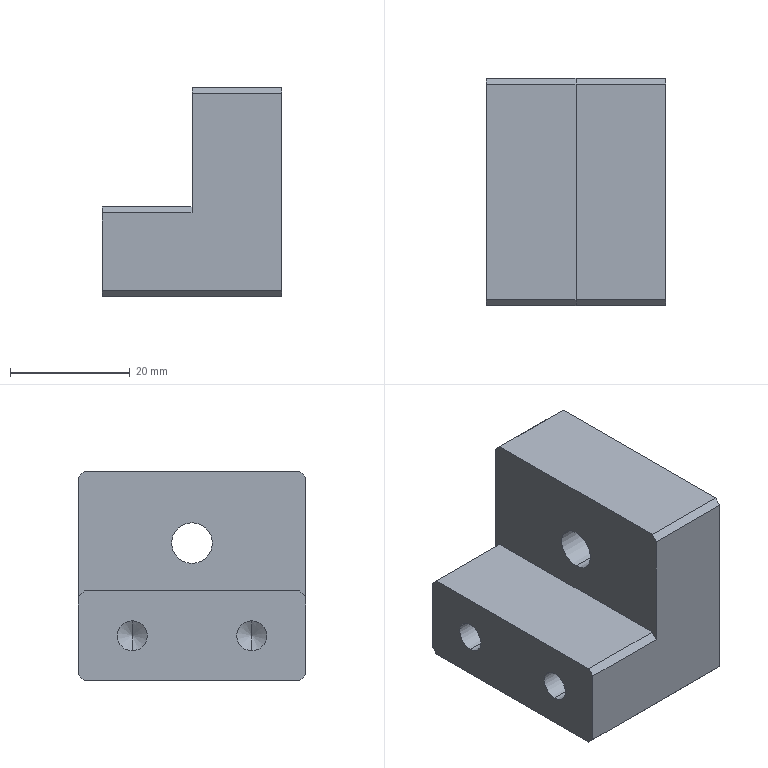Part | SolidWorks | features BaseBody 1 | 1 solid | 27 faces | box 30 x 38 x 35 mm | volume 26589 mm3 | plane 15 | cylinder 8 | cone 4 | commonest cylinder face diameters 5 x4 6.8 x2 18.5 x2
STEP:
#1=CARTESIAN_POINT('',(15.,0.,26.4));
#2=VERTEX_POINT('',#1);
#3=CARTESIAN_POINT('',(15.,0.,19.6));
#4=VERTEX_POINT('',#3);
#5=CARTESIAN_POINT('',(15.,0.,23.));
#6=DIRECTION('',(1.,0.,0.));
#7=DIRECTION('',(0.,0.,-1.));
#8=AXIS2_PLACEMENT_3D('',#5,#6,#7);
#9=CIRCLE('',#8,3.4);
#10=EDGE_CURVE('',#2,#4,#9,.T.);
#11=ORIENTED_EDGE('',*,*,#10,.F.);
#12=CARTESIAN_POINT('',(27.,0.,26.4));
#13=VERTEX_POINT('',#12);
#14=CARTESIAN_POINT('',(27.,0.,26.4));
#15=DIRECTION('',(1.,0.,0.));
#16=VECTOR('',#15,1000.);
#17=LINE('',#14,#16);
#18=EDGE_CURVE('',#2,#13,#17,.T.);
#19=ORIENTED_EDGE('',*,*,#18,.T.);
#20=CARTESIAN_POINT('',(27.,0.,19.6));
#21=VERTEX_POINT('',#20);
#22=CARTESIAN_POINT('',(27.,0.,23.));
#23=DIRECTION('',(1.,0.,0.));
#24=DIRECTION('',(0.,0.,-1.));
#25=AXIS2_PLACEMENT_3D('',#22,#23,#24);
#26=CIRCLE('',#25,3.4);
#27=EDGE_CURVE('',#13,#21,#26,.T.);
#28=ORIENTED_EDGE('',*,*,#27,.T.);
#29=CARTESIAN_POINT('',(27.,0.,19.6));
#30=DIRECTION('',(1.,0.,0.));
#31=VECTOR('',#30,1000.);
#32=LINE('',#29,#31);
#33=EDGE_CURVE('',#4,#21,#32,.T.);
#34=ORIENTED_EDGE('',*,*,#33,.F.);
#35=EDGE_LOOP('',(#11,#19,#28,#34));
#36=FACE_OUTER_BOUND('',#35,.T.);
#37=CARTESIAN_POINT('',(27.,0.,23.));
#38=DIRECTION('',(1.,0.,0.));
#39=DIRECTION('',(0.,0.,-1.));
#40=AXIS2_PLACEMENT_3D('',#37,#38,#39);
#41=CYLINDRICAL_SURFACE('',#40,3.4);
#42=ADVANCED_FACE('',(#36),#41,.F.);
#43=CARTESIAN_POINT('',(27.,0.,32.25));
#44=VERTEX_POINT('',#43);
#45=CARTESIAN_POINT('',(27.,0.,13.75));
#46=VERTEX_POINT('',#45);
#47=CARTESIAN_POINT('',(27.,0.,23.));
#48=DIRECTION('',(1.,0.,0.));
#49=DIRECTION('',(0.,0.,-1.));
#50=AXIS2_PLACEMENT_3D('',#47,#48,#49);
#51=CIRCLE('',#50,9.25);
#52=EDGE_CURVE('',#44,#46,#51,.T.);
#53=ORIENTED_EDGE('',*,*,#52,.F.);
#54=CARTESIAN_POINT('',(30.,0.,32.25));
#55=VERTEX_POINT('',#54);
#56=CARTESIAN_POINT('',(27.,0.,32.25));
#57=DIRECTION('',(1.,0.,0.));
#58=VECTOR('',#57,1000.);
#59=LINE('',#56,#58);
#60=EDGE_CURVE('',#44,#55,#59,.T.);
#61=ORIENTED_EDGE('',*,*,#60,.T.);
#62=CARTESIAN_POINT('',(30.,0.,13.75));
#63=VERTEX_POINT('',#62);
#64=CARTESIAN_POINT('',(30.,0.,23.));
#65=DIRECTION('',(1.,0.,0.));
#66=DIRECTION('',(0.,0.,-1.));
#67=AXIS2_PLACEMENT_3D('',#64,#65,#66);
#68=CIRCLE('',#67,9.25);
#69=EDGE_CURVE('',#55,#63,#68,.T.);
#70=ORIENTED_EDGE('',*,*,#69,.T.);
#71=CARTESIAN_POINT('',(27.,0.,13.75));
#72=DIRECTION('',(1.,0.,0.));
#73=VECTOR('',#72,1000.);
#74=LINE('',#71,#73);
#75=EDGE_CURVE('',#46,#63,#74,.T.);
#76=ORIENTED_EDGE('',*,*,#75,.F.);
#77=EDGE_LOOP('',(#53,#61,#70,#76));
#78=FACE_OUTER_BOUND('',#77,.T.);
#79=CARTESIAN_POINT('',(27.,0.,23.));
#80=DIRECTION('',(1.,0.,0.));
#81=DIRECTION('',(0.,0.,-1.));
#82=AXIS2_PLACEMENT_3D('',#79,#80,#81);
#83=CYLINDRICAL_SURFACE('',#82,9.25);
#84=ADVANCED_FACE('',(#78),#83,.F.);
#85=CARTESIAN_POINT('',(15.,10.,5.));
#86=VERTEX_POINT('',#85);
#87=CARTESIAN_POINT('',(15.,10.,10.));
#88=VERTEX_POINT('',#87);
#89=CARTESIAN_POINT('',(15.,10.,7.5));
#90=DIRECTION('',(-1.,0.,0.));
#91=DIRECTION('',(0.,0.,1.));
#92=AXIS2_PLACEMENT_3D('',#89,#90,#91);
#93=CIRCLE('',#92,2.5);
#94=EDGE_CURVE('',#86,#88,#93,.T.);
#95=ORIENTED_EDGE('',*,*,#94,.F.);
#96=CARTESIAN_POINT('',(0.,10.,5.));
#97=VERTEX_POINT('',#96);
#98=CARTESIAN_POINT('',(0.,10.,5.));
#99=DIRECTION('',(-1.,0.,0.));
#100=VECTOR('',#99,1000.);
#101=LINE('',#98,#100);
#102=EDGE_CURVE('',#86,#97,#101,.T.);
#103=ORIENTED_EDGE('',*,*,#102,.T.);
#104=CARTESIAN_POINT('',(0.,10.,10.));
#105=VERTEX_POINT('',#104);
#106=CARTESIAN_POINT('',(0.,10.,7.5));
#107=DIRECTION('',(-1.,0.,0.));
#108=DIRECTION('',(0.,0.,1.));
#109=AXIS2_PLACEMENT_3D('',#106,#107,#108);
#110=CIRCLE('',#109,2.5);
#111=EDGE_CURVE('',#97,#105,#110,.T.);
#112=ORIENTED_EDGE('',*,*,#111,.T.);
#113=CARTESIAN_POINT('',(0.,10.,10.));
#114=DIRECTION('',(-1.,0.,0.));
#115=VECTOR('',#114,1000.);
#116=LINE('',#113,#115);
#117=EDGE_CURVE('',#88,#105,#116,.T.);
#118=ORIENTED_EDGE('',*,*,#117,.F.);
#119=EDGE_LOOP('',(#95,#103,#112,#118));
#120=FACE_OUTER_BOUND('',#119,.T.);
#121=CARTESIAN_POINT('',(0.,10.,7.5));
#122=DIRECTION('',(-1.,0.,0.));
#123=DIRECTION('',(0.,0.,1.));
#124=AXIS2_PLACEMENT_3D('',#121,#122,#123);
#125=CYLINDRICAL_SURFACE('',#124,2.5);
#126=ADVANCED_FACE('',(#120),#125,.F.);
#127=CARTESIAN_POINT('',(16.502,10.,7.5));
#128=VERTEX_POINT('',#127);
#129=CARTESIAN_POINT('',(15.,10.,10.));
#130=DIRECTION('',(-0.515,0.,0.8572));
#131=VECTOR('',#130,1000.);
#132=LINE('',#129,#131);
#133=EDGE_CURVE('',#128,#88,#132,.T.);
#134=ORIENTED_EDGE('',*,*,#133,.F.);
#135=CARTESIAN_POINT('',(15.,10.,5.));
#136=DIRECTION('',(-0.515,0.,-0.8572));
#137=VECTOR('',#136,1000.);
#138=LINE('',#135,#137);
#139=EDGE_CURVE('',#128,#86,#138,.T.);
#140=ORIENTED_EDGE('',*,*,#139,.T.);
#141=ORIENTED_EDGE('',*,*,#94,.T.);
#142=EDGE_LOOP('',(#134,#140,#141));
#143=FACE_OUTER_BOUND('',#142,.T.);
#144=CARTESIAN_POINT('',(15.,10.,7.5));
#145=DIRECTION('',(-1.,0.,0.));
#146=DIRECTION('',(0.,0.,1.));
#147=AXIS2_PLACEMENT_3D('',#144,#145,#146);
#148=CONICAL_SURFACE('',#147,2.5,1.03);
#149=ADVANCED_FACE('',(#143),#148,.F.);
#150=CARTESIAN_POINT('',(15.,-10.,5.));
#151=VERTEX_POINT('',#150);
#152=CARTESIAN_POINT('',(15.,-10.,10.));
#153=VERTEX_POINT('',#152);
#154=CARTESIAN_POINT('',(15.,-10.,7.5));
#155=DIRECTION('',(-1.,0.,0.));
#156=DIRECTION('',(0.,0.,1.));
#157=AXIS2_PLACEMENT_3D('',#154,#155,#156);
#158=CIRCLE('',#157,2.5);
#159=EDGE_CURVE('',#151,#153,#158,.T.);
#160=ORIENTED_EDGE('',*,*,#159,.F.);
#161=CARTESIAN_POINT('',(0.,-10.,5.));
#162=VERTEX_POINT('',#161);
#163=CARTESIAN_POINT('',(0.,-10.,5.));
#164=DIRECTION('',(-1.,0.,0.));
#165=VECTOR('',#164,1000.);
#166=LINE('',#163,#165);
#167=EDGE_CURVE('',#151,#162,#166,.T.);
#168=ORIENTED_EDGE('',*,*,#167,.T.);
#169=CARTESIAN_POINT('',(0.,-10.,10.));
#170=VERTEX_POINT('',#169);
#171=CARTESIAN_POINT('',(0.,-10.,7.5));
#172=DIRECTION('',(-1.,0.,0.));
#173=DIRECTION('',(0.,0.,1.));
#174=AXIS2_PLACEMENT_3D('',#171,#172,#173);
#175=CIRCLE('',#174,2.5);
#176=EDGE_CURVE('',#162,#170,#175,.T.);
#177=ORIENTED_EDGE('',*,*,#176,.T.);
#178=CARTESIAN_POINT('',(0.,-10.,10.));
#179=DIRECTION('',(-1.,0.,0.));
#180=VECTOR('',#179,1000.);
#181=LINE('',#178,#180);
#182=EDGE_CURVE('',#153,#170,#181,.T.);
#183=ORIENTED_EDGE('',*,*,#182,.F.);
#184=EDGE_LOOP('',(#160,#168,#177,#183));
#185=FACE_OUTER_BOUND('',#184,.T.);
#186=CARTESIAN_POINT('',(0.,-10.,7.5));
#187=DIRECTION('',(-1.,0.,0.));
#188=DIRECTION('',(0.,0.,1.));
#189=AXIS2_PLACEMENT_3D('',#186,#187,#188);
#190=CYLINDRICAL_SURFACE('',#189,2.5);
#191=ADVANCED_FACE('',(#185),#190,.F.);
#192=CARTESIAN_POINT('',(16.502,-10.,7.5));
#193=VERTEX_POINT('',#192);
#194=CARTESIAN_POINT('',(15.,-10.,10.));
#195=DIRECTION('',(-0.515,0.,0.8572));
#196=VECTOR('',#195,1000.);
#197=LINE('',#194,#196);
#198=EDGE_CURVE('',#193,#153,#197,.T.);
#199=ORIENTED_EDGE('',*,*,#198,.F.);
#200=CARTESIAN_POINT('',(15.,-10.,5.));
#201=DIRECTION('',(-0.515,0.,-0.8572));
#202=VECTOR('',#201,1000.);
#203=LINE('',#200,#202);
#204=EDGE_CURVE('',#193,#151,#203,.T.);
#205=ORIENTED_EDGE('',*,*,#204,.T.);
#206=ORIENTED_EDGE('',*,*,#159,.T.);
#207=EDGE_LOOP('',(#199,#205,#206));
#208=FACE_OUTER_BOUND('',#207,.T.);
#209=CARTESIAN_POINT('',(15.,-10.,7.5));
#210=DIRECTION('',(-1.,0.,0.));
#211=DIRECTION('',(0.,0.,1.));
#212=AXIS2_PLACEMENT_3D('',#209,#210,#211);
#213=CONICAL_SURFACE('',#212,2.5,1.03);
#214=ADVANCED_FACE('',(#208),#213,.F.);
#215=CARTESIAN_POINT('',(15.,18.,35.));
#216=VERTEX_POINT('',#215);
#217=CARTESIAN_POINT('',(15.,19.,34.));
#218=VERTEX_POINT('',#217);
#219=CARTESIAN_POINT('',(15.,19.,34.));
#220=DIRECTION('',(0.,0.7071,-0.7071));
#221=VECTOR('',#220,1000.);
#222=LINE('',#219,#221);
#223=EDGE_CURVE('',#216,#218,#222,.T.);
#224=ORIENTED_EDGE('',*,*,#223,.F.);
#225=CARTESIAN_POINT('',(30.,18.,35.));
#226=VERTEX_POINT('',#225);
#227=CARTESIAN_POINT('',(30.,18.,35.));
#228=DIRECTION('',(-1.,0.,0.));
#229=VECTOR('',#228,1000.);
#230=LINE('',#227,#229);
#231=EDGE_CURVE('',#226,#216,#230,.T.);
#232=ORIENTED_EDGE('',*,*,#231,.F.);
#233=CARTESIAN_POINT('',(30.,19.,34.));
#234=VERTEX_POINT('',#233);
#235=CARTESIAN_POINT('',(30.,19.,34.));
#236=DIRECTION('',(0.,-0.7071,0.7071));
#237=VECTOR('',#236,1000.);
#238=LINE('',#235,#237);
#239=EDGE_CURVE('',#234,#226,#238,.T.);
#240=ORIENTED_EDGE('',*,*,#239,.F.);
#241=CARTESIAN_POINT('',(0.,19.,34.));
#242=DIRECTION('',(1.,0.,0.));
#243=VECTOR('',#242,1000.);
#244=LINE('',#241,#243);
#245=EDGE_CURVE('',#218,#234,#244,.T.);
#246=ORIENTED_EDGE('',*,*,#245,.F.);
#247=EDGE_LOOP('',(#224,#232,#240,#246));
#248=FACE_OUTER_BOUND('',#247,.T.);
#249=CARTESIAN_POINT('',(0.,19.,34.));
#250=DIRECTION('',(0.,-0.7071,-0.7071));
#251=DIRECTION('',(0.,-0.7071,0.7071));
#252=AXIS2_PLACEMENT_3D('',#249,#250,#251);
#253=PLANE('',#252);
#254=ADVANCED_FACE('',(#248),#253,.F.);
#255=CARTESIAN_POINT('',(15.,-19.,34.));
#256=VERTEX_POINT('',#255);
#257=CARTESIAN_POINT('',(15.,-18.,35.));
#258=VERTEX_POINT('',#257);
#259=CARTESIAN_POINT('',(15.,-18.,35.));
#260=DIRECTION('',(0.,0.7071,0.7071));
#261=VECTOR('',#260,1000.);
#262=LINE('',#259,#261);
#263=EDGE_CURVE('',#256,#258,#262,.T.);
#264=ORIENTED_EDGE('',*,*,#263,.F.);
#265=CARTESIAN_POINT('',(30.,-19.,34.));
#266=VERTEX_POINT('',#265);
#267=CARTESIAN_POINT('',(15.,-19.,34.));
#268=DIRECTION('',(-1.,0.,0.));
#269=VECTOR('',#268,1000.);
#270=LINE('',#267,#269);
#271=EDGE_CURVE('',#266,#256,#270,.T.);
#272=ORIENTED_EDGE('',*,*,#271,.F.);
#273=CARTESIAN_POINT('',(30.,-18.,35.));
#274=VERTEX_POINT('',#273);
#275=CARTESIAN_POINT('',(30.,-18.,35.));
#276=DIRECTION('',(0.,-0.7071,-0.7071));
#277=VECTOR('',#276,1000.);
#278=LINE('',#275,#277);
#279=EDGE_CURVE('',#274,#266,#278,.T.);
#280=ORIENTED_EDGE('',*,*,#279,.F.);
#281=CARTESIAN_POINT('',(30.,-18.,35.));
#282=DIRECTION('',(1.,0.,0.));
#283=VECTOR('',#282,1000.);
#284=LINE('',#281,#283);
#285=EDGE_CURVE('',#258,#274,#284,.T.);
#286=ORIENTED_EDGE('',*,*,#285,.F.);
#287=EDGE_LOOP('',(#264,#272,#280,#286));
#288=FACE_OUTER_BOUND('',#287,.T.);
#289=CARTESIAN_POINT('',(30.,-18.,35.));
#290=DIRECTION('',(0.,-0.7071,0.7071));
#291=DIRECTION('',(-1.,0.,0.));
#292=AXIS2_PLACEMENT_3D('',#289,#290,#291);
#293=PLANE('',#292);
#294=ADVANCED_FACE('',(#288),#293,.T.);
#295=CARTESIAN_POINT('',(30.,18.,0.));
#296=VERTEX_POINT('',#295);
#297=CARTESIAN_POINT('',(30.,19.,1.));
#298=VERTEX_POINT('',#297);
#299=CARTESIAN_POINT('',(30.,19.,1.));
#300=DIRECTION('',(0.,0.7071,0.7071));
#301=VECTOR('',#300,1000.);
#302=LINE('',#299,#301);
#303=EDGE_CURVE('',#296,#298,#302,.T.);
#304=ORIENTED_EDGE('',*,*,#303,.F.);
#305=CARTESIAN_POINT('',(0.,18.,0.));
#306=VERTEX_POINT('',#305);
#307=CARTESIAN_POINT('',(0.,18.,0.));
#308=DIRECTION('',(1.,0.,0.));
#309=VECTOR('',#308,1000.);
#310=LINE('',#307,#309);
#311=EDGE_CURVE('',#306,#296,#310,.T.);
#312=ORIENTED_EDGE('',*,*,#311,.F.);
#313=CARTESIAN_POINT('',(0.,19.,1.));
#314=VERTEX_POINT('',#313);
#315=CARTESIAN_POINT('',(0.,19.,1.));
#316=DIRECTION('',(0.,-0.7071,-0.7071));
#317=VECTOR('',#316,1000.);
#318=LINE('',#315,#317);
#319=EDGE_CURVE('',#314,#306,#318,.T.);
#320=ORIENTED_EDGE('',*,*,#319,.F.);
#321=CARTESIAN_POINT('',(0.,19.,1.));
#322=DIRECTION('',(-1.,0.,0.));
#323=VECTOR('',#322,1000.);
#324=LINE('',#321,#323);
#325=EDGE_CURVE('',#298,#314,#324,.T.);
#326=ORIENTED_EDGE('',*,*,#325,.F.);
#327=EDGE_LOOP('',(#304,#312,#320,#326));
#328=FACE_OUTER_BOUND('',#327,.T.);
#329=CARTESIAN_POINT('',(0.,19.,1.));
#330=DIRECTION('',(0.,-0.7071,0.7071));
#331=DIRECTION('',(-1.,0.,0.));
#332=AXIS2_PLACEMENT_3D('',#329,#330,#331);
#333=PLANE('',#332);
#334=ADVANCED_FACE('',(#328),#333,.F.);
#335=CARTESIAN_POINT('',(30.,-19.,1.));
#336=VERTEX_POINT('',#335);
#337=CARTESIAN_POINT('',(30.,-18.,0.));
#338=VERTEX_POINT('',#337);
#339=CARTESIAN_POINT('',(30.,-18.,0.));
#340=DIRECTION('',(0.,0.7071,-0.7071));
#341=VECTOR('',#340,1000.);
#342=LINE('',#339,#341);
#343=EDGE_CURVE('',#336,#338,#342,.T.);
#344=ORIENTED_EDGE('',*,*,#343,.F.);
#345=CARTESIAN_POINT('',(0.,-19.,1.));
#346=VERTEX_POINT('',#345);
#347=CARTESIAN_POINT('',(30.,-19.,1.));
#348=DIRECTION('',(1.,0.,0.));
#349=VECTOR('',#348,1000.);
#350=LINE('',#347,#349);
#351=EDGE_CURVE('',#346,#336,#350,.T.);
#352=ORIENTED_EDGE('',*,*,#351,.F.);
#353=CARTESIAN_POINT('',(0.,-18.,0.));
#354=VERTEX_POINT('',#353);
#355=CARTESIAN_POINT('',(0.,-18.,0.));
#356=DIRECTION('',(0.,-0.7071,0.7071));
#357=VECTOR('',#356,1000.);
#358=LINE('',#355,#357);
#359=EDGE_CURVE('',#354,#346,#358,.T.);
#360=ORIENTED_EDGE('',*,*,#359,.F.);
#361=CARTESIAN_POINT('',(0.,-18.,0.));
#362=DIRECTION('',(-1.,0.,0.));
#363=VECTOR('',#362,1000.);
#364=LINE('',#361,#363);
#365=EDGE_CURVE('',#338,#354,#364,.T.);
#366=ORIENTED_EDGE('',*,*,#365,.F.);
#367=EDGE_LOOP('',(#344,#352,#360,#366));
#368=FACE_OUTER_BOUND('',#367,.T.);
#369=CARTESIAN_POINT('',(0.,-18.,0.));
#370=DIRECTION('',(0.,-0.7071,-0.7071));
#371=DIRECTION('',(0.,-0.7071,0.7071));
#372=AXIS2_PLACEMENT_3D('',#369,#370,#371);
#373=PLANE('',#372);
#374=ADVANCED_FACE('',(#368),#373,.T.);
#375=CARTESIAN_POINT('',(0.,-19.,14.));
#376=VERTEX_POINT('',#375);
#377=CARTESIAN_POINT('',(0.,-18.,15.));
#378=VERTEX_POINT('',#377);
#379=CARTESIAN_POINT('',(0.,-18.,15.));
#380=DIRECTION('',(0.,0.7071,0.7071));
#381=VECTOR('',#380,1000.);
#382=LINE('',#379,#381);
#383=EDGE_CURVE('',#376,#378,#382,.T.);
#384=ORIENTED_EDGE('',*,*,#383,.F.);
#385=CARTESIAN_POINT('',(15.,-19.,14.));
#386=VERTEX_POINT('',#385);
#387=CARTESIAN_POINT('',(0.,-19.,14.));
#388=DIRECTION('',(-1.,0.,0.));
#389=VECTOR('',#388,1000.);
#390=LINE('',#387,#389);
#391=EDGE_CURVE('',#386,#376,#390,.T.);
#392=ORIENTED_EDGE('',*,*,#391,.F.);
#393=CARTESIAN_POINT('',(15.,-18.,15.));
#394=VERTEX_POINT('',#393);
#395=CARTESIAN_POINT('',(15.,10.5,43.5));
#396=DIRECTION('',(0.,-0.7071,-0.7071));
#397=VECTOR('',#396,1000.);
#398=LINE('',#395,#397);
#399=EDGE_CURVE('',#394,#386,#398,.T.);
#400=ORIENTED_EDGE('',*,*,#399,.F.);
#401=CARTESIAN_POINT('',(15.,-18.,15.));
#402=DIRECTION('',(1.,0.,0.));
#403=VECTOR('',#402,1000.);
#404=LINE('',#401,#403);
#405=EDGE_CURVE('',#378,#394,#404,.T.);
#406=ORIENTED_EDGE('',*,*,#405,.F.);
#407=EDGE_LOOP('',(#384,#392,#400,#406));
#408=FACE_OUTER_BOUND('',#407,.T.);
#409=CARTESIAN_POINT('',(15.,-18.,15.));
#410=DIRECTION('',(0.,-0.7071,0.7071));
#411=DIRECTION('',(-1.,0.,0.));
#412=AXIS2_PLACEMENT_3D('',#409,#410,#411);
#413=PLANE('',#412);
#414=ADVANCED_FACE('',(#408),#413,.T.);
#415=CARTESIAN_POINT('',(0.,18.,15.));
#416=VERTEX_POINT('',#415);
#417=CARTESIAN_POINT('',(0.,19.,14.));
#418=VERTEX_POINT('',#417);
#419=CARTESIAN_POINT('',(0.,19.,14.));
#420=DIRECTION('',(0.,0.7071,-0.7071));
#421=VECTOR('',#420,1000.);
#422=LINE('',#419,#421);
#423=EDGE_CURVE('',#416,#418,#422,.T.);
#424=ORIENTED_EDGE('',*,*,#423,.F.);
#425=CARTESIAN_POINT('',(15.,18.,15.));
#426=VERTEX_POINT('',#425);
#427=CARTESIAN_POINT('',(15.,18.,15.));
#428=DIRECTION('',(-1.,0.,0.));
#429=VECTOR('',#428,1000.);
#430=LINE('',#427,#429);
#431=EDGE_CURVE('',#426,#416,#430,.T.);
#432=ORIENTED_EDGE('',*,*,#431,.F.);
#433=CARTESIAN_POINT('',(15.,19.,14.));
#434=VERTEX_POINT('',#433);
#435=CARTESIAN_POINT('',(15.,8.5,24.5));
#436=DIRECTION('',(0.,-0.7071,0.7071));
#437=VECTOR('',#436,1000.);
#438=LINE('',#435,#437);
#439=EDGE_CURVE('',#434,#426,#438,.T.);
#440=ORIENTED_EDGE('',*,*,#439,.F.);
#441=CARTESIAN_POINT('',(0.,19.,14.));
#442=DIRECTION('',(1.,0.,0.));
#443=VECTOR('',#442,1000.);
#444=LINE('',#441,#443);
#445=EDGE_CURVE('',#418,#434,#444,.T.);
#446=ORIENTED_EDGE('',*,*,#445,.F.);
#447=EDGE_LOOP('',(#424,#432,#440,#446));
#448=FACE_OUTER_BOUND('',#447,.T.);
#449=CARTESIAN_POINT('',(0.,19.,14.));
#450=DIRECTION('',(0.,-0.7071,-0.7071));
#451=DIRECTION('',(0.,-0.7071,0.7071));
#452=AXIS2_PLACEMENT_3D('',#449,#450,#451);
#453=PLANE('',#452);
#454=ADVANCED_FACE('',(#448),#453,.F.);
#455=CARTESIAN_POINT('',(27.,0.,23.));
#456=DIRECTION('',(1.,0.,0.));
#457=DIRECTION('',(0.,0.,-1.));
#458=AXIS2_PLACEMENT_3D('',#455,#456,#457);
#459=CIRCLE('',#458,3.4);
#460=EDGE_CURVE('',#21,#13,#459,.T.);
#461=ORIENTED_EDGE('',*,*,#460,.F.);
#462=ORIENTED_EDGE('',*,*,#27,.F.);
#463=EDGE_LOOP('',(#461,#462));
#464=FACE_BOUND('',#463,.T.);
#465=CARTESIAN_POINT('',(27.,0.,23.));
#466=DIRECTION('',(1.,0.,0.));
#467=DIRECTION('',(0.,0.,-1.));
#468=AXIS2_PLACEMENT_3D('',#465,#466,#467);
#469=CIRCLE('',#468,9.25);
#470=EDGE_CURVE('',#46,#44,#469,.T.);
#471=ORIENTED_EDGE('',*,*,#470,.T.);
#472=ORIENTED_EDGE('',*,*,#52,.T.);
#473=EDGE_LOOP('',(#471,#472));
#474=FACE_OUTER_BOUND('',#473,.T.);
#475=CARTESIAN_POINT('',(27.,0.,23.));
#476=DIRECTION('',(1.,0.,0.));
#477=DIRECTION('',(0.,0.,-1.));
#478=AXIS2_PLACEMENT_3D('',#475,#476,#477);
#479=PLANE('',#478);
#480=ADVANCED_FACE('',(#464,#474),#479,.T.);
#481=CARTESIAN_POINT('',(15.,-19.,35.));
#482=DIRECTION('',(0.,0.,1.));
#483=VECTOR('',#482,1000.);
#484=LINE('',#481,#483);
#485=EDGE_CURVE('',#386,#256,#484,.T.);
#486=ORIENTED_EDGE('',*,*,#485,.F.);
#487=ORIENTED_EDGE('',*,*,#391,.T.);
#488=CARTESIAN_POINT('',(0.,-19.,15.));
#489=DIRECTION('',(0.,0.,1.));
#490=VECTOR('',#489,1000.);
#491=LINE('',#488,#490);
#492=EDGE_CURVE('',#346,#376,#491,.T.);
#493=ORIENTED_EDGE('',*,*,#492,.F.);
#494=ORIENTED_EDGE('',*,*,#351,.T.);
#495=CARTESIAN_POINT('',(30.,-19.,0.));
#496=DIRECTION('',(0.,0.,-1.));
#497=VECTOR('',#496,1000.);
#498=LINE('',#495,#497);
#499=EDGE_CURVE('',#266,#336,#498,.T.);
#500=ORIENTED_EDGE('',*,*,#499,.F.);
#501=ORIENTED_EDGE('',*,*,#271,.T.);
#502=EDGE_LOOP('',(#486,#487,#493,#494,#500,#501));
#503=FACE_OUTER_BOUND('',#502,.T.);
#504=CARTESIAN_POINT('',(0.,-19.,0.));
#505=DIRECTION('',(0.,-1.,0.));
#506=DIRECTION('',(0.,0.,-1.));
#507=AXIS2_PLACEMENT_3D('',#504,#505,#506);
#508=PLANE('',#507);
#509=ADVANCED_FACE('',(#503),#508,.T.);
#510=CARTESIAN_POINT('',(0.,19.,15.));
#511=DIRECTION('',(0.,0.,1.));
#512=VECTOR('',#511,1000.);
#513=LINE('',#510,#512);
#514=EDGE_CURVE('',#314,#418,#513,.T.);
#515=ORIENTED_EDGE('',*,*,#514,.T.);
#516=ORIENTED_EDGE('',*,*,#445,.T.);
#517=CARTESIAN_POINT('',(15.,19.,35.));
#518=DIRECTION('',(0.,0.,1.));
#519=VECTOR('',#518,1000.);
#520=LINE('',#517,#519);
#521=EDGE_CURVE('',#434,#218,#520,.T.);
#522=ORIENTED_EDGE('',*,*,#521,.T.);
#523=ORIENTED_EDGE('',*,*,#245,.T.);
#524=CARTESIAN_POINT('',(30.,19.,0.));
#525=DIRECTION('',(0.,0.,-1.));
#526=VECTOR('',#525,1000.);
#527=LINE('',#524,#526);
#528=EDGE_CURVE('',#234,#298,#527,.T.);
#529=ORIENTED_EDGE('',*,*,#528,.T.);
#530=ORIENTED_EDGE('',*,*,#325,.T.);
#531=EDGE_LOOP('',(#515,#516,#522,#523,#529,#530));
#532=FACE_OUTER_BOUND('',#531,.T.);
#533=CARTESIAN_POINT('',(0.,19.,0.));
#534=DIRECTION('',(0.,-1.,0.));
#535=DIRECTION('',(0.,0.,-1.));
#536=AXIS2_PLACEMENT_3D('',#533,#534,#535);
#537=PLANE('',#536);
#538=ADVANCED_FACE('',(#532),#537,.F.);
#539=CARTESIAN_POINT('',(30.,19.,0.));
#540=DIRECTION('',(0.,-1.,0.));
#541=VECTOR('',#540,1000.);
#542=LINE('',#539,#541);
#543=EDGE_CURVE('',#296,#338,#542,.T.);
#544=ORIENTED_EDGE('',*,*,#543,.T.);
#545=ORIENTED_EDGE('',*,*,#365,.T.);
#546=CARTESIAN_POINT('',(0.,19.,0.));
#547=DIRECTION('',(0.,-1.,0.));
#548=VECTOR('',#547,1000.);
#549=LINE('',#546,#548);
#550=EDGE_CURVE('',#306,#354,#549,.T.);
#551=ORIENTED_EDGE('',*,*,#550,.F.);
#552=ORIENTED_EDGE('',*,*,#311,.T.);
#553=EDGE_LOOP('',(#544,#545,#551,#552));
#554=FACE_OUTER_BOUND('',#553,.T.);
#555=CARTESIAN_POINT('',(0.,19.,0.));
#556=DIRECTION('',(0.,0.,1.));
#557=DIRECTION('',(1.,0.,0.));
#558=AXIS2_PLACEMENT_3D('',#555,#556,#557);
#559=PLANE('',#558);
#560=ADVANCED_FACE('',(#554),#559,.F.);
#561=CARTESIAN_POINT('',(30.,0.,23.));
#562=DIRECTION('',(1.,0.,0.));
#563=DIRECTION('',(0.,0.,-1.));
#564=AXIS2_PLACEMENT_3D('',#561,#562,#563);
#565=CIRCLE('',#564,9.25);
#566=EDGE_CURVE('',#63,#55,#565,.T.);
#567=ORIENTED_EDGE('',*,*,#566,.F.);
#568=ORIENTED_EDGE('',*,*,#69,.F.);
#569=EDGE_LOOP('',(#567,#568));
#570=FACE_BOUND('',#569,.T.);
#571=ORIENTED_EDGE('',*,*,#499,.T.);
#572=ORIENTED_EDGE('',*,*,#343,.T.);
#573=ORIENTED_EDGE('',*,*,#543,.F.);
#574=ORIENTED_EDGE('',*,*,#303,.T.);
#575=ORIENTED_EDGE('',*,*,#528,.F.);
#576=ORIENTED_EDGE('',*,*,#239,.T.);
#577=CARTESIAN_POINT('',(30.,19.,35.));
#578=DIRECTION('',(0.,-1.,0.));
#579=VECTOR('',#578,1000.);
#580=LINE('',#577,#579);
#581=EDGE_CURVE('',#226,#274,#580,.T.);
#582=ORIENTED_EDGE('',*,*,#581,.T.);
#583=ORIENTED_EDGE('',*,*,#279,.T.);
#584=EDGE_LOOP('',(#571,#572,#573,#574,#575,#576,#582,#583));
#585=FACE_OUTER_BOUND('',#584,.T.);
#586=CARTESIAN_POINT('',(30.,19.,0.));
#587=DIRECTION('',(-1.,0.,0.));
#588=DIRECTION('',(0.,1.,0.));
#589=AXIS2_PLACEMENT_3D('',#586,#587,#588);
#590=PLANE('',#589);
#591=ADVANCED_FACE('',(#570,#585),#590,.F.);
#592=CARTESIAN_POINT('',(15.,19.,35.));
#593=DIRECTION('',(0.,-1.,0.));
#594=VECTOR('',#593,1000.);
#595=LINE('',#592,#594);
#596=EDGE_CURVE('',#216,#258,#595,.T.);
#597=ORIENTED_EDGE('',*,*,#596,.T.);
#598=ORIENTED_EDGE('',*,*,#285,.T.);
#599=ORIENTED_EDGE('',*,*,#581,.F.);
#600=ORIENTED_EDGE('',*,*,#231,.T.);
#601=EDGE_LOOP('',(#597,#598,#599,#600));
#602=FACE_OUTER_BOUND('',#601,.T.);
#603=CARTESIAN_POINT('',(30.,19.,35.));
#604=DIRECTION('',(0.,0.,-1.));
#605=DIRECTION('',(0.,-1.,0.));
#606=AXIS2_PLACEMENT_3D('',#603,#604,#605);
#607=PLANE('',#606);
#608=ADVANCED_FACE('',(#602),#607,.F.);
#609=CARTESIAN_POINT('',(15.,0.,23.));
#610=DIRECTION('',(1.,0.,0.));
#611=DIRECTION('',(0.,0.,-1.));
#612=AXIS2_PLACEMENT_3D('',#609,#610,#611);
#613=CIRCLE('',#612,3.4);
#614=EDGE_CURVE('',#4,#2,#613,.T.);
#615=ORIENTED_EDGE('',*,*,#614,.T.);
#616=ORIENTED_EDGE('',*,*,#10,.T.);
#617=EDGE_LOOP('',(#615,#616));
#618=FACE_BOUND('',#617,.T.);
#619=ORIENTED_EDGE('',*,*,#485,.T.);
#620=ORIENTED_EDGE('',*,*,#263,.T.);
#621=ORIENTED_EDGE('',*,*,#596,.F.);
#622=ORIENTED_EDGE('',*,*,#223,.T.);
#623=ORIENTED_EDGE('',*,*,#521,.F.);
#624=ORIENTED_EDGE('',*,*,#439,.T.);
#625=CARTESIAN_POINT('',(15.,19.,15.));
#626=DIRECTION('',(0.,-1.,0.));
#627=VECTOR('',#626,1000.);
#628=LINE('',#625,#627);
#629=EDGE_CURVE('',#426,#394,#628,.T.);
#630=ORIENTED_EDGE('',*,*,#629,.T.);
#631=ORIENTED_EDGE('',*,*,#399,.T.);
#632=EDGE_LOOP('',(#619,#620,#621,#622,#623,#624,#630,#631));
#633=FACE_OUTER_BOUND('',#632,.T.);
#634=CARTESIAN_POINT('',(15.,19.,35.));
#635=DIRECTION('',(1.,0.,0.));
#636=DIRECTION('',(0.,0.,1.));
#637=AXIS2_PLACEMENT_3D('',#634,#635,#636);
#638=PLANE('',#637);
#639=ADVANCED_FACE('',(#618,#633),#638,.F.);
#640=ORIENTED_EDGE('',*,*,#629,.F.);
#641=ORIENTED_EDGE('',*,*,#431,.T.);
#642=CARTESIAN_POINT('',(0.,19.,15.));
#643=DIRECTION('',(0.,-1.,0.));
#644=VECTOR('',#643,1000.);
#645=LINE('',#642,#644);
#646=EDGE_CURVE('',#416,#378,#645,.T.);
#647=ORIENTED_EDGE('',*,*,#646,.T.);
#648=ORIENTED_EDGE('',*,*,#405,.T.);
#649=EDGE_LOOP('',(#640,#641,#647,#648));
#650=FACE_OUTER_BOUND('',#649,.T.);
#651=CARTESIAN_POINT('',(15.,19.,15.));
#652=DIRECTION('',(0.,0.,-1.));
#653=DIRECTION('',(-1.,0.,0.));
#654=AXIS2_PLACEMENT_3D('',#651,#652,#653);
#655=PLANE('',#654);
#656=ADVANCED_FACE('',(#650),#655,.F.);
#657=CARTESIAN_POINT('',(0.,-10.,7.5));
#658=DIRECTION('',(-1.,0.,0.));
#659=DIRECTION('',(0.,0.,1.));
#660=AXIS2_PLACEMENT_3D('',#657,#658,#659);
#661=CIRCLE('',#660,2.5);
#662=EDGE_CURVE('',#170,#162,#661,.T.);
#663=ORIENTED_EDGE('',*,*,#662,.F.);
#664=ORIENTED_EDGE('',*,*,#176,.F.);
#665=EDGE_LOOP('',(#663,#664));
#666=FACE_BOUND('',#665,.T.);
#667=CARTESIAN_POINT('',(0.,10.,7.5));
#668=DIRECTION('',(-1.,0.,0.));
#669=DIRECTION('',(0.,0.,1.));
#670=AXIS2_PLACEMENT_3D('',#667,#668,#669);
#671=CIRCLE('',#670,2.5);
#672=EDGE_CURVE('',#105,#97,#671,.T.);
#673=ORIENTED_EDGE('',*,*,#672,.F.);
#674=ORIENTED_EDGE('',*,*,#111,.F.);
#675=EDGE_LOOP('',(#673,#674));
#676=FACE_BOUND('',#675,.T.);
#677=ORIENTED_EDGE('',*,*,#646,.F.);
#678=ORIENTED_EDGE('',*,*,#423,.T.);
#679=ORIENTED_EDGE('',*,*,#514,.F.);
#680=ORIENTED_EDGE('',*,*,#319,.T.);
#681=ORIENTED_EDGE('',*,*,#550,.T.);
#682=ORIENTED_EDGE('',*,*,#359,.T.);
#683=ORIENTED_EDGE('',*,*,#492,.T.);
#684=ORIENTED_EDGE('',*,*,#383,.T.);
#685=EDGE_LOOP('',(#677,#678,#679,#680,#681,#682,#683,#684));
#686=FACE_OUTER_BOUND('',#685,.T.);
#687=CARTESIAN_POINT('',(0.,19.,15.));
#688=DIRECTION('',(1.,0.,0.));
#689=DIRECTION('',(0.,1.,0.));
#690=AXIS2_PLACEMENT_3D('',#687,#688,#689);
#691=PLANE('',#690);
#692=ADVANCED_FACE('',(#666,#676,#686),#691,.F.);
#693=ORIENTED_EDGE('',*,*,#204,.F.);
#694=ORIENTED_EDGE('',*,*,#198,.T.);
#695=CARTESIAN_POINT('',(15.,-10.,7.5));
#696=DIRECTION('',(-1.,0.,0.));
#697=DIRECTION('',(0.,0.,1.));
#698=AXIS2_PLACEMENT_3D('',#695,#696,#697);
#699=CIRCLE('',#698,2.5);
#700=EDGE_CURVE('',#153,#151,#699,.T.);
#701=ORIENTED_EDGE('',*,*,#700,.T.);
#702=EDGE_LOOP('',(#693,#694,#701));
#703=FACE_OUTER_BOUND('',#702,.T.);
#704=CARTESIAN_POINT('',(15.,-10.,7.5));
#705=DIRECTION('',(-1.,0.,0.));
#706=DIRECTION('',(0.,0.,1.));
#707=AXIS2_PLACEMENT_3D('',#704,#705,#706);
#708=CONICAL_SURFACE('',#707,2.5,1.03);
#709=ADVANCED_FACE('',(#703),#708,.F.);
#710=ORIENTED_EDGE('',*,*,#167,.F.);
#711=ORIENTED_EDGE('',*,*,#700,.F.);
#712=ORIENTED_EDGE('',*,*,#182,.T.);
#713=ORIENTED_EDGE('',*,*,#662,.T.);
#714=EDGE_LOOP('',(#710,#711,#712,#713));
#715=FACE_OUTER_BOUND('',#714,.T.);
#716=CARTESIAN_POINT('',(0.,-10.,7.5));
#717=DIRECTION('',(-1.,0.,0.));
#718=DIRECTION('',(0.,0.,1.));
#719=AXIS2_PLACEMENT_3D('',#716,#717,#718);
#720=CYLINDRICAL_SURFACE('',#719,2.5);
#721=ADVANCED_FACE('',(#715),#720,.F.);
#722=ORIENTED_EDGE('',*,*,#139,.F.);
#723=ORIENTED_EDGE('',*,*,#133,.T.);
#724=CARTESIAN_POINT('',(15.,10.,7.5));
#725=DIRECTION('',(-1.,0.,0.));
#726=DIRECTION('',(0.,0.,1.));
#727=AXIS2_PLACEMENT_3D('',#724,#725,#726);
#728=CIRCLE('',#727,2.5);
#729=EDGE_CURVE('',#88,#86,#728,.T.);
#730=ORIENTED_EDGE('',*,*,#729,.T.);
#731=EDGE_LOOP('',(#722,#723,#730));
#732=FACE_OUTER_BOUND('',#731,.T.);
#733=CARTESIAN_POINT('',(15.,10.,7.5));
#734=DIRECTION('',(-1.,0.,0.));
#735=DIRECTION('',(0.,0.,1.));
#736=AXIS2_PLACEMENT_3D('',#733,#734,#735);
#737=CONICAL_SURFACE('',#736,2.5,1.03);
#738=ADVANCED_FACE('',(#732),#737,.F.);
#739=ORIENTED_EDGE('',*,*,#102,.F.);
#740=ORIENTED_EDGE('',*,*,#729,.F.);
#741=ORIENTED_EDGE('',*,*,#117,.T.);
#742=ORIENTED_EDGE('',*,*,#672,.T.);
#743=EDGE_LOOP('',(#739,#740,#741,#742));
#744=FACE_OUTER_BOUND('',#743,.T.);
#745=CARTESIAN_POINT('',(0.,10.,7.5));
#746=DIRECTION('',(-1.,0.,0.));
#747=DIRECTION('',(0.,0.,1.));
#748=AXIS2_PLACEMENT_3D('',#745,#746,#747);
#749=CYLINDRICAL_SURFACE('',#748,2.5);
#750=ADVANCED_FACE('',(#744),#749,.F.);
#751=ORIENTED_EDGE('',*,*,#60,.F.);
#752=ORIENTED_EDGE('',*,*,#470,.F.);
#753=ORIENTED_EDGE('',*,*,#75,.T.);
#754=ORIENTED_EDGE('',*,*,#566,.T.);
#755=EDGE_LOOP('',(#751,#752,#753,#754));
#756=FACE_OUTER_BOUND('',#755,.T.);
#757=CARTESIAN_POINT('',(27.,0.,23.));
#758=DIRECTION('',(1.,0.,0.));
#759=DIRECTION('',(0.,0.,-1.));
#760=AXIS2_PLACEMENT_3D('',#757,#758,#759);
#761=CYLINDRICAL_SURFACE('',#760,9.25);
#762=ADVANCED_FACE('',(#756),#761,.F.);
#763=ORIENTED_EDGE('',*,*,#18,.F.);
#764=ORIENTED_EDGE('',*,*,#614,.F.);
#765=ORIENTED_EDGE('',*,*,#33,.T.);
#766=ORIENTED_EDGE('',*,*,#460,.T.);
#767=EDGE_LOOP('',(#763,#764,#765,#766));
#768=FACE_OUTER_BOUND('',#767,.T.);
#769=CARTESIAN_POINT('',(27.,0.,23.));
#770=DIRECTION('',(1.,0.,0.));
#771=DIRECTION('',(0.,0.,-1.));
#772=AXIS2_PLACEMENT_3D('',#769,#770,#771);
#773=CYLINDRICAL_SURFACE('',#772,3.4);
#774=ADVANCED_FACE('',(#768),#773,.F.);
#775=CLOSED_SHELL('',(#42,#84,#126,#149,#191,#214,#254,#294,#334,#374,#414,#454,#480,#509,#538,#560,#591,#608,#639,#656,#692,#709,#721,#738,#750,#762,#774));
#776=MANIFOLD_SOLID_BREP('',#775);
#777=CARTESIAN_POINT('',(0.,0.,0.));
#778=DIRECTION('',(0.,0.,1.));
#779=DIRECTION('',(1.,0.,0.));
#780=AXIS2_PLACEMENT_3D('',#777,#778,#779);
#781=(LENGTH_UNIT()NAMED_UNIT(*)SI_UNIT(.MILLI.,.METRE.));
#782=UNCERTAINTY_MEASURE_WITH_UNIT(LENGTH_MEASURE(0.00001),#781,'','');
#783=(NAMED_UNIT(*)PLANE_ANGLE_UNIT()SI_UNIT($,.RADIAN.));
#784=(NAMED_UNIT(*)SI_UNIT($,.STERADIAN.)SOLID_ANGLE_UNIT());
#785=(GEOMETRIC_REPRESENTATION_CONTEXT(3)GLOBAL_UNCERTAINTY_ASSIGNED_CONTEXT((#782))GLOBAL_UNIT_ASSIGNED_CONTEXT((#781,#783,#784))REPRESENTATION_CONTEXT('',''));
#786=ADVANCED_BREP_SHAPE_REPRESENTATION('',(#776,#780),#785);